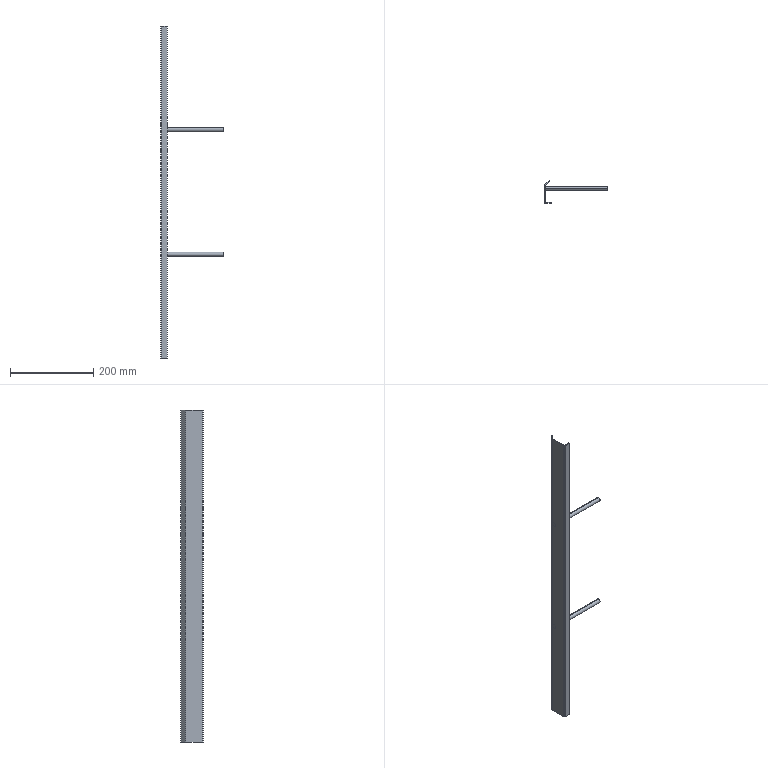Part | STEP file | MM-P41130-12_1 | 1 solid | 20 faces | box 151.5 x 53.167 x 800 mm | volume 109265 mm3 | plane 12 | cylinder 8 | commonest cylinder face diameters 10 x4 1.473 x2 4.473 x2
STEP:
#1=CARTESIAN_POINT('',(0.,0.,0.));
#2=DIRECTION('',(0.,0.,1.));
#3=DIRECTION('',(1.,0.,0.));
#4=AXIS2_PLACEMENT_3D('',#1,#2,#3);
#5=CARTESIAN_POINT('',(0.,-16.5,-145.));
#6=VERTEX_POINT('',#5);
#7=CARTESIAN_POINT('',(0.,-16.5,-155.));
#8=VERTEX_POINT('',#7);
#9=CARTESIAN_POINT('',(0.,-16.5,-150.));
#10=DIRECTION('',(-1.,0.,0.));
#11=DIRECTION('',(0.,0.,-1.));
#12=AXIS2_PLACEMENT_3D('',#9,#10,#11);
#13=CIRCLE('',#12,5.);
#14=CARTESIAN_POINT('',(150.,-16.5,-150.));
#15=DIRECTION('',(1.,0.,0.));
#16=DIRECTION('',(0.,0.,-1.));
#17=AXIS2_PLACEMENT_3D('',#14,#15,#16);
#18=CYLINDRICAL_SURFACE('',#17,5.);
#19=CARTESIAN_POINT('',(6.283,-150.));
#20=DIRECTION('',(-1.,0.));
#21=VECTOR('',#20,1.);
#22=LINE('',#19,#21);
#23=(GEOMETRIC_REPRESENTATION_CONTEXT(2)PARAMETRIC_REPRESENTATION_CONTEXT()REPRESENTATION_CONTEXT('',''));
#24=DEFINITIONAL_REPRESENTATION('',(#22),#23);
#25=PCURVE('',#18,#24);
#26=CARTESIAN_POINT('',(0.,-50.,-400.));
#27=DIRECTION('',(1.,0.,0.));
#28=DIRECTION('',(0.,0.,-1.));
#29=AXIS2_PLACEMENT_3D('',#26,#27,#28);
#30=PLANE('',#29);
#31=CARTESIAN_POINT('',(-245.,33.5));
#32=CARTESIAN_POINT('',(-245.,24.84));
#33=CARTESIAN_POINT('',(-252.5,29.17));
#34=CARTESIAN_POINT('',(-260.,33.5));
#35=CARTESIAN_POINT('',(-252.5,37.83));
#36=CARTESIAN_POINT('',(-245.,42.16));
#37=CARTESIAN_POINT('',(-245.,33.5));
#38=(BOUNDED_CURVE()B_SPLINE_CURVE(2,(#31,#32,#33,#34,#35,#36,#37),.UNSPECIFIED.,.T.,.F.)B_SPLINE_CURVE_WITH_KNOTS((1,2,2,2,2,1),(-2.094,0.,2.094,4.189,6.283,8.378),.UNSPECIFIED.)CURVE()GEOMETRIC_REPRESENTATION_ITEM()RATIONAL_B_SPLINE_CURVE((1.,0.5,1.,0.5,1.,0.5,1.))REPRESENTATION_ITEM(''));
#39=(GEOMETRIC_REPRESENTATION_CONTEXT(2)PARAMETRIC_REPRESENTATION_CONTEXT()REPRESENTATION_CONTEXT('',''));
#40=DEFINITIONAL_REPRESENTATION('',(#38),#39);
#41=PCURVE('',#30,#40);
#42=SURFACE_CURVE('',#13,(#25,#41),.PCURVE_S1.);
#43=EDGE_CURVE('',#6,#8,#42,.T.);
#44=ORIENTED_EDGE('',*,*,#43,.F.);
#45=CARTESIAN_POINT('',(150.,-16.5,-145.));
#46=VERTEX_POINT('',#45);
#47=CARTESIAN_POINT('',(150.,-16.5,-145.));
#48=DIRECTION('',(1.,0.,0.));
#49=VECTOR('',#48,1.);
#50=LINE('',#47,#49);
#51=CARTESIAN_POINT('',(3.142,0.));
#52=DIRECTION('',(0.,1.));
#53=VECTOR('',#52,1.);
#54=LINE('',#51,#53);
#55=(GEOMETRIC_REPRESENTATION_CONTEXT(2)PARAMETRIC_REPRESENTATION_CONTEXT()REPRESENTATION_CONTEXT('',''));
#56=DEFINITIONAL_REPRESENTATION('',(#54),#55);
#57=PCURVE('',#18,#56);
#58=CARTESIAN_POINT('',(150.,-16.5,-150.));
#59=DIRECTION('',(1.,0.,0.));
#60=DIRECTION('',(0.,0.,-1.));
#61=AXIS2_PLACEMENT_3D('',#58,#59,#60);
#62=CYLINDRICAL_SURFACE('',#61,5.);
#63=CARTESIAN_POINT('',(3.142,0.));
#64=DIRECTION('',(0.,1.));
#65=VECTOR('',#64,1.);
#66=LINE('',#63,#65);
#67=(GEOMETRIC_REPRESENTATION_CONTEXT(2)PARAMETRIC_REPRESENTATION_CONTEXT()REPRESENTATION_CONTEXT('',''));
#68=DEFINITIONAL_REPRESENTATION('',(#66),#67);
#69=PCURVE('',#62,#68);
#70=SURFACE_CURVE('',#50,(#57,#69),.PCURVE_S1.);
#71=EDGE_CURVE('',#6,#46,#70,.T.);
#72=ORIENTED_EDGE('',*,*,#71,.T.);
#73=CARTESIAN_POINT('',(150.,-16.5,-155.));
#74=VERTEX_POINT('',#73);
#75=CARTESIAN_POINT('',(150.,-16.5,-150.));
#76=DIRECTION('',(-1.,0.,0.));
#77=DIRECTION('',(0.,0.,-1.));
#78=AXIS2_PLACEMENT_3D('',#75,#76,#77);
#79=CIRCLE('',#78,5.);
#80=CARTESIAN_POINT('',(6.283,0.));
#81=DIRECTION('',(-1.,0.));
#82=VECTOR('',#81,1.);
#83=LINE('',#80,#82);
#84=(GEOMETRIC_REPRESENTATION_CONTEXT(2)PARAMETRIC_REPRESENTATION_CONTEXT()REPRESENTATION_CONTEXT('',''));
#85=DEFINITIONAL_REPRESENTATION('',(#83),#84);
#86=PCURVE('',#18,#85);
#87=CARTESIAN_POINT('',(150.,-16.5,-150.));
#88=DIRECTION('',(1.,0.,0.));
#89=DIRECTION('',(0.,1.,0.));
#90=AXIS2_PLACEMENT_3D('',#87,#88,#89);
#91=PLANE('',#90);
#92=CARTESIAN_POINT('',(0.,-5.));
#93=CARTESIAN_POINT('',(-8.66,-5.));
#94=CARTESIAN_POINT('',(-4.33,2.5));
#95=CARTESIAN_POINT('',(0.,10.));
#96=CARTESIAN_POINT('',(4.33,2.5));
#97=CARTESIAN_POINT('',(8.66,-5.));
#98=CARTESIAN_POINT('',(0.,-5.));
#99=(BOUNDED_CURVE()B_SPLINE_CURVE(2,(#92,#93,#94,#95,#96,#97,#98),.UNSPECIFIED.,.T.,.F.)B_SPLINE_CURVE_WITH_KNOTS((1,2,2,2,2,1),(-2.094,0.,2.094,4.189,6.283,8.378),.UNSPECIFIED.)CURVE()GEOMETRIC_REPRESENTATION_ITEM()RATIONAL_B_SPLINE_CURVE((1.,0.5,1.,0.5,1.,0.5,1.))REPRESENTATION_ITEM(''));
#100=(GEOMETRIC_REPRESENTATION_CONTEXT(2)PARAMETRIC_REPRESENTATION_CONTEXT()REPRESENTATION_CONTEXT('',''));
#101=DEFINITIONAL_REPRESENTATION('',(#99),#100);
#102=PCURVE('',#91,#101);
#103=SURFACE_CURVE('',#79,(#86,#102),.PCURVE_S1.);
#104=EDGE_CURVE('',#46,#74,#103,.T.);
#105=ORIENTED_EDGE('',*,*,#104,.T.);
#106=CARTESIAN_POINT('',(150.,-16.5,-155.));
#107=DIRECTION('',(1.,0.,0.));
#108=VECTOR('',#107,1.);
#109=LINE('',#106,#108);
#110=CARTESIAN_POINT('',(0.,0.));
#111=DIRECTION('',(0.,1.));
#112=VECTOR('',#111,1.);
#113=LINE('',#110,#112);
#114=(GEOMETRIC_REPRESENTATION_CONTEXT(2)PARAMETRIC_REPRESENTATION_CONTEXT()REPRESENTATION_CONTEXT('',''));
#115=DEFINITIONAL_REPRESENTATION('',(#113),#114);
#116=PCURVE('',#18,#115);
#117=CARTESIAN_POINT('',(6.283,0.));
#118=DIRECTION('',(0.,1.));
#119=VECTOR('',#118,1.);
#120=LINE('',#117,#119);
#121=(GEOMETRIC_REPRESENTATION_CONTEXT(2)PARAMETRIC_REPRESENTATION_CONTEXT()REPRESENTATION_CONTEXT('',''));
#122=DEFINITIONAL_REPRESENTATION('',(#120),#121);
#123=PCURVE('',#62,#122);
#124=SURFACE_CURVE('',#109,(#116,#123),.PCURVE_S1.);
#125=EDGE_CURVE('',#8,#74,#124,.T.);
#126=ORIENTED_EDGE('',*,*,#125,.F.);
#127=EDGE_LOOP('',(#44,#72,#105,#126));
#128=FACE_BOUND('',#127,.T.);
#129=ADVANCED_FACE('',(#128),#18,.T.);
#130=CARTESIAN_POINT('',(0.,-16.5,155.));
#131=VERTEX_POINT('',#130);
#132=CARTESIAN_POINT('',(0.,-16.5,145.));
#133=VERTEX_POINT('',#132);
#134=CARTESIAN_POINT('',(0.,-16.5,150.));
#135=DIRECTION('',(-1.,0.,0.));
#136=DIRECTION('',(0.,0.,-1.));
#137=AXIS2_PLACEMENT_3D('',#134,#135,#136);
#138=CIRCLE('',#137,5.);
#139=CARTESIAN_POINT('',(150.,-16.5,150.));
#140=DIRECTION('',(1.,0.,0.));
#141=DIRECTION('',(0.,0.,-1.));
#142=AXIS2_PLACEMENT_3D('',#139,#140,#141);
#143=CYLINDRICAL_SURFACE('',#142,5.);
#144=CARTESIAN_POINT('',(6.283,-150.));
#145=DIRECTION('',(-1.,0.));
#146=VECTOR('',#145,1.);
#147=LINE('',#144,#146);
#148=(GEOMETRIC_REPRESENTATION_CONTEXT(2)PARAMETRIC_REPRESENTATION_CONTEXT()REPRESENTATION_CONTEXT('',''));
#149=DEFINITIONAL_REPRESENTATION('',(#147),#148);
#150=PCURVE('',#143,#149);
#151=CARTESIAN_POINT('',(-545.,33.5));
#152=CARTESIAN_POINT('',(-545.,24.84));
#153=CARTESIAN_POINT('',(-552.5,29.17));
#154=CARTESIAN_POINT('',(-560.,33.5));
#155=CARTESIAN_POINT('',(-552.5,37.83));
#156=CARTESIAN_POINT('',(-545.,42.16));
#157=CARTESIAN_POINT('',(-545.,33.5));
#158=(BOUNDED_CURVE()B_SPLINE_CURVE(2,(#151,#152,#153,#154,#155,#156,#157),.UNSPECIFIED.,.T.,.F.)B_SPLINE_CURVE_WITH_KNOTS((1,2,2,2,2,1),(-2.094,0.,2.094,4.189,6.283,8.378),.UNSPECIFIED.)CURVE()GEOMETRIC_REPRESENTATION_ITEM()RATIONAL_B_SPLINE_CURVE((1.,0.5,1.,0.5,1.,0.5,1.))REPRESENTATION_ITEM(''));
#159=(GEOMETRIC_REPRESENTATION_CONTEXT(2)PARAMETRIC_REPRESENTATION_CONTEXT()REPRESENTATION_CONTEXT('',''));
#160=DEFINITIONAL_REPRESENTATION('',(#158),#159);
#161=PCURVE('',#30,#160);
#162=SURFACE_CURVE('',#138,(#150,#161),.PCURVE_S1.);
#163=EDGE_CURVE('',#131,#133,#162,.T.);
#164=ORIENTED_EDGE('',*,*,#163,.F.);
#165=CARTESIAN_POINT('',(150.,-16.5,155.));
#166=VERTEX_POINT('',#165);
#167=CARTESIAN_POINT('',(150.,-16.5,155.));
#168=DIRECTION('',(1.,0.,0.));
#169=VECTOR('',#168,1.);
#170=LINE('',#167,#169);
#171=CARTESIAN_POINT('',(3.142,0.));
#172=DIRECTION('',(0.,1.));
#173=VECTOR('',#172,1.);
#174=LINE('',#171,#173);
#175=(GEOMETRIC_REPRESENTATION_CONTEXT(2)PARAMETRIC_REPRESENTATION_CONTEXT()REPRESENTATION_CONTEXT('',''));
#176=DEFINITIONAL_REPRESENTATION('',(#174),#175);
#177=PCURVE('',#143,#176);
#178=CARTESIAN_POINT('',(150.,-16.5,150.));
#179=DIRECTION('',(1.,0.,0.));
#180=DIRECTION('',(0.,0.,-1.));
#181=AXIS2_PLACEMENT_3D('',#178,#179,#180);
#182=CYLINDRICAL_SURFACE('',#181,5.);
#183=CARTESIAN_POINT('',(3.142,0.));
#184=DIRECTION('',(0.,1.));
#185=VECTOR('',#184,1.);
#186=LINE('',#183,#185);
#187=(GEOMETRIC_REPRESENTATION_CONTEXT(2)PARAMETRIC_REPRESENTATION_CONTEXT()REPRESENTATION_CONTEXT('',''));
#188=DEFINITIONAL_REPRESENTATION('',(#186),#187);
#189=PCURVE('',#182,#188);
#190=SURFACE_CURVE('',#170,(#177,#189),.PCURVE_S1.);
#191=EDGE_CURVE('',#131,#166,#190,.T.);
#192=ORIENTED_EDGE('',*,*,#191,.T.);
#193=CARTESIAN_POINT('',(150.,-16.5,145.));
#194=VERTEX_POINT('',#193);
#195=CARTESIAN_POINT('',(150.,-16.5,150.));
#196=DIRECTION('',(-1.,0.,0.));
#197=DIRECTION('',(0.,0.,-1.));
#198=AXIS2_PLACEMENT_3D('',#195,#196,#197);
#199=CIRCLE('',#198,5.);
#200=CARTESIAN_POINT('',(6.283,0.));
#201=DIRECTION('',(-1.,0.));
#202=VECTOR('',#201,1.);
#203=LINE('',#200,#202);
#204=(GEOMETRIC_REPRESENTATION_CONTEXT(2)PARAMETRIC_REPRESENTATION_CONTEXT()REPRESENTATION_CONTEXT('',''));
#205=DEFINITIONAL_REPRESENTATION('',(#203),#204);
#206=PCURVE('',#143,#205);
#207=CARTESIAN_POINT('',(150.,-16.5,150.));
#208=DIRECTION('',(1.,0.,0.));
#209=DIRECTION('',(0.,1.,0.));
#210=AXIS2_PLACEMENT_3D('',#207,#208,#209);
#211=PLANE('',#210);
#212=CARTESIAN_POINT('',(0.,-5.));
#213=CARTESIAN_POINT('',(-8.66,-5.));
#214=CARTESIAN_POINT('',(-4.33,2.5));
#215=CARTESIAN_POINT('',(0.,10.));
#216=CARTESIAN_POINT('',(4.33,2.5));
#217=CARTESIAN_POINT('',(8.66,-5.));
#218=CARTESIAN_POINT('',(0.,-5.));
#219=(BOUNDED_CURVE()B_SPLINE_CURVE(2,(#212,#213,#214,#215,#216,#217,#218),.UNSPECIFIED.,.T.,.F.)B_SPLINE_CURVE_WITH_KNOTS((1,2,2,2,2,1),(-2.094,0.,2.094,4.189,6.283,8.378),.UNSPECIFIED.)CURVE()GEOMETRIC_REPRESENTATION_ITEM()RATIONAL_B_SPLINE_CURVE((1.,0.5,1.,0.5,1.,0.5,1.))REPRESENTATION_ITEM(''));
#220=(GEOMETRIC_REPRESENTATION_CONTEXT(2)PARAMETRIC_REPRESENTATION_CONTEXT()REPRESENTATION_CONTEXT('',''));
#221=DEFINITIONAL_REPRESENTATION('',(#219),#220);
#222=PCURVE('',#211,#221);
#223=SURFACE_CURVE('',#199,(#206,#222),.PCURVE_S1.);
#224=EDGE_CURVE('',#166,#194,#223,.T.);
#225=ORIENTED_EDGE('',*,*,#224,.T.);
#226=CARTESIAN_POINT('',(150.,-16.5,145.));
#227=DIRECTION('',(1.,0.,0.));
#228=VECTOR('',#227,1.);
#229=LINE('',#226,#228);
#230=CARTESIAN_POINT('',(0.,0.));
#231=DIRECTION('',(0.,1.));
#232=VECTOR('',#231,1.);
#233=LINE('',#230,#232);
#234=(GEOMETRIC_REPRESENTATION_CONTEXT(2)PARAMETRIC_REPRESENTATION_CONTEXT()REPRESENTATION_CONTEXT('',''));
#235=DEFINITIONAL_REPRESENTATION('',(#233),#234);
#236=PCURVE('',#143,#235);
#237=CARTESIAN_POINT('',(6.283,0.));
#238=DIRECTION('',(0.,1.));
#239=VECTOR('',#238,1.);
#240=LINE('',#237,#239);
#241=(GEOMETRIC_REPRESENTATION_CONTEXT(2)PARAMETRIC_REPRESENTATION_CONTEXT()REPRESENTATION_CONTEXT('',''));
#242=DEFINITIONAL_REPRESENTATION('',(#240),#241);
#243=PCURVE('',#182,#242);
#244=SURFACE_CURVE('',#229,(#236,#243),.PCURVE_S1.);
#245=EDGE_CURVE('',#133,#194,#244,.T.);
#246=ORIENTED_EDGE('',*,*,#245,.F.);
#247=EDGE_LOOP('',(#164,#192,#225,#246));
#248=FACE_BOUND('',#247,.T.);
#249=ADVANCED_FACE('',(#248),#143,.T.);
#250=CARTESIAN_POINT('',(-1.5,-10.305,-400.));
#251=VERTEX_POINT('',#250);
#252=CARTESIAN_POINT('',(-1.5,-10.305,400.));
#253=VERTEX_POINT('',#252);
#254=CARTESIAN_POINT('',(-1.5,-10.305,-400.));
#255=DIRECTION('',(0.,0.,1.));
#256=VECTOR('',#255,1.);
#257=LINE('',#254,#256);
#258=CARTESIAN_POINT('',(-1.5,-50.,-400.));
#259=DIRECTION('',(1.,0.,0.));
#260=DIRECTION('',(0.,0.,-1.));
#261=AXIS2_PLACEMENT_3D('',#258,#259,#260);
#262=PLANE('',#261);
#263=CARTESIAN_POINT('',(0.,39.695));
#264=DIRECTION('',(-1.,0.));
#265=VECTOR('',#264,1.);
#266=LINE('',#263,#265);
#267=(GEOMETRIC_REPRESENTATION_CONTEXT(2)PARAMETRIC_REPRESENTATION_CONTEXT()REPRESENTATION_CONTEXT('',''));
#268=DEFINITIONAL_REPRESENTATION('',(#266),#267);
#269=PCURVE('',#262,#268);
#270=CARTESIAN_POINT('',(0.7366,-10.305,-400.));
#271=DIRECTION('',(0.,0.,-1.));
#272=DIRECTION('',(-1.,0.,0.));
#273=AXIS2_PLACEMENT_3D('',#270,#271,#272);
#274=CYLINDRICAL_SURFACE('',#273,2.237);
#275=CARTESIAN_POINT('',(0.,0.));
#276=DIRECTION('',(0.,-1.));
#277=VECTOR('',#276,1.);
#278=LINE('',#275,#277);
#279=(GEOMETRIC_REPRESENTATION_CONTEXT(2)PARAMETRIC_REPRESENTATION_CONTEXT()REPRESENTATION_CONTEXT('',''));
#280=DEFINITIONAL_REPRESENTATION('',(#278),#279);
#281=PCURVE('',#274,#280);
#282=SURFACE_CURVE('',#257,(#269,#281),.PCURVE_S1.);
#283=EDGE_CURVE('',#251,#253,#282,.T.);
#284=ORIENTED_EDGE('',*,*,#283,.F.);
#285=CARTESIAN_POINT('',(-1.5,-49.263,-400.));
#286=VERTEX_POINT('',#285);
#287=CARTESIAN_POINT('',(-1.5,-50.,-400.));
#288=DIRECTION('',(0.,1.,0.));
#289=VECTOR('',#288,1.);
#290=LINE('',#287,#289);
#291=CARTESIAN_POINT('',(0.,0.));
#292=DIRECTION('',(0.,1.));
#293=VECTOR('',#292,1.);
#294=LINE('',#291,#293);
#295=(GEOMETRIC_REPRESENTATION_CONTEXT(2)PARAMETRIC_REPRESENTATION_CONTEXT()REPRESENTATION_CONTEXT('',''));
#296=DEFINITIONAL_REPRESENTATION('',(#294),#295);
#297=PCURVE('',#262,#296);
#298=CARTESIAN_POINT('',(0.,-49.263,-400.));
#299=DIRECTION('',(0.,0.,-1.));
#300=DIRECTION('',(-1.,0.,0.));
#301=AXIS2_PLACEMENT_3D('',#298,#299,#300);
#302=PLANE('',#301);
#303=CARTESIAN_POINT('',(1.5,-0.7366));
#304=DIRECTION('',(0.,1.));
#305=VECTOR('',#304,1.);
#306=LINE('',#303,#305);
#307=(GEOMETRIC_REPRESENTATION_CONTEXT(2)PARAMETRIC_REPRESENTATION_CONTEXT()REPRESENTATION_CONTEXT('',''));
#308=DEFINITIONAL_REPRESENTATION('',(#306),#307);
#309=PCURVE('',#302,#308);
#310=SURFACE_CURVE('',#290,(#297,#309),.PCURVE_S1.);
#311=EDGE_CURVE('',#286,#251,#310,.T.);
#312=ORIENTED_EDGE('',*,*,#311,.F.);
#313=CARTESIAN_POINT('',(-1.5,-49.263,400.));
#314=VERTEX_POINT('',#313);
#315=CARTESIAN_POINT('',(-1.5,-49.263,-400.));
#316=DIRECTION('',(0.,0.,-1.));
#317=VECTOR('',#316,1.);
#318=LINE('',#315,#317);
#319=CARTESIAN_POINT('',(0.,0.7366));
#320=DIRECTION('',(1.,0.));
#321=VECTOR('',#320,1.);
#322=LINE('',#319,#321);
#323=(GEOMETRIC_REPRESENTATION_CONTEXT(2)PARAMETRIC_REPRESENTATION_CONTEXT()REPRESENTATION_CONTEXT('',''));
#324=DEFINITIONAL_REPRESENTATION('',(#322),#323);
#325=PCURVE('',#262,#324);
#326=CARTESIAN_POINT('',(0.7366,-49.263,-400.));
#327=DIRECTION('',(0.,0.,-1.));
#328=DIRECTION('',(-1.,0.,0.));
#329=AXIS2_PLACEMENT_3D('',#326,#327,#328);
#330=CYLINDRICAL_SURFACE('',#329,2.237);
#331=CARTESIAN_POINT('',(6.283,0.));
#332=DIRECTION('',(0.,1.));
#333=VECTOR('',#332,1.);
#334=LINE('',#331,#333);
#335=(GEOMETRIC_REPRESENTATION_CONTEXT(2)PARAMETRIC_REPRESENTATION_CONTEXT()REPRESENTATION_CONTEXT('',''));
#336=DEFINITIONAL_REPRESENTATION('',(#334),#335);
#337=PCURVE('',#330,#336);
#338=SURFACE_CURVE('',#318,(#325,#337),.PCURVE_S1.);
#339=EDGE_CURVE('',#314,#286,#338,.T.);
#340=ORIENTED_EDGE('',*,*,#339,.F.);
#341=CARTESIAN_POINT('',(-1.5,-50.,400.));
#342=DIRECTION('',(0.,-1.,0.));
#343=VECTOR('',#342,1.);
#344=LINE('',#341,#343);
#345=CARTESIAN_POINT('',(-800.,0.));
#346=DIRECTION('',(0.,-1.));
#347=VECTOR('',#346,1.);
#348=LINE('',#345,#347);
#349=(GEOMETRIC_REPRESENTATION_CONTEXT(2)PARAMETRIC_REPRESENTATION_CONTEXT()REPRESENTATION_CONTEXT('',''));
#350=DEFINITIONAL_REPRESENTATION('',(#348),#349);
#351=PCURVE('',#262,#350);
#352=CARTESIAN_POINT('',(0.,-10.305,400.));
#353=DIRECTION('',(0.,0.,1.));
#354=DIRECTION('',(1.,0.,0.));
#355=AXIS2_PLACEMENT_3D('',#352,#353,#354);
#356=PLANE('',#355);
#357=CARTESIAN_POINT('',(-1.5,-39.695));
#358=DIRECTION('',(0.,-1.));
#359=VECTOR('',#358,1.);
#360=LINE('',#357,#359);
#361=(GEOMETRIC_REPRESENTATION_CONTEXT(2)PARAMETRIC_REPRESENTATION_CONTEXT()REPRESENTATION_CONTEXT('',''));
#362=DEFINITIONAL_REPRESENTATION('',(#360),#361);
#363=PCURVE('',#356,#362);
#364=SURFACE_CURVE('',#344,(#351,#363),.PCURVE_S1.);
#365=EDGE_CURVE('',#253,#314,#364,.T.);
#366=ORIENTED_EDGE('',*,*,#365,.F.);
#367=EDGE_LOOP('',(#284,#312,#340,#366));
#368=FACE_BOUND('',#367,.T.);
#369=ADVANCED_FACE('',(#368),#262,.F.);
#370=CARTESIAN_POINT('',(10.607,0.6066,400.));
#371=VERTEX_POINT('',#370);
#372=CARTESIAN_POINT('',(9.546,1.667,400.));
#373=VERTEX_POINT('',#372);
#374=CARTESIAN_POINT('',(9.546,1.667,400.));
#375=DIRECTION('',(-0.7071,0.7071,0.));
#376=VECTOR('',#375,1.);
#377=LINE('',#374,#376);
#378=CARTESIAN_POINT('',(9.546,11.972));
#379=DIRECTION('',(-0.7071,0.7071));
#380=VECTOR('',#379,1.);
#381=LINE('',#378,#380);
#382=(GEOMETRIC_REPRESENTATION_CONTEXT(2)PARAMETRIC_REPRESENTATION_CONTEXT()REPRESENTATION_CONTEXT('',''));
#383=DEFINITIONAL_REPRESENTATION('',(#381),#382);
#384=PCURVE('',#356,#383);
#385=CARTESIAN_POINT('',(9.546,1.667,-400.));
#386=DIRECTION('',(-0.7071,-0.7071,0.));
#387=DIRECTION('',(0.7071,-0.7071,0.));
#388=AXIS2_PLACEMENT_3D('',#385,#386,#387);
#389=PLANE('',#388);
#390=CARTESIAN_POINT('',(0.,800.));
#391=DIRECTION('',(-1.,0.));
#392=VECTOR('',#391,1.);
#393=LINE('',#390,#392);
#394=(GEOMETRIC_REPRESENTATION_CONTEXT(2)PARAMETRIC_REPRESENTATION_CONTEXT()REPRESENTATION_CONTEXT('',''));
#395=DEFINITIONAL_REPRESENTATION('',(#393),#394);
#396=PCURVE('',#389,#395);
#397=SURFACE_CURVE('',#377,(#384,#396),.PCURVE_S1.);
#398=EDGE_CURVE('',#371,#373,#397,.T.);
#399=ORIENTED_EDGE('',*,*,#398,.T.);
#400=CARTESIAN_POINT('',(-0.8449,-8.724,400.));
#401=VERTEX_POINT('',#400);
#402=CARTESIAN_POINT('',(9.546,1.667,400.));
#403=DIRECTION('',(-0.7071,-0.7071,0.));
#404=VECTOR('',#403,1.);
#405=LINE('',#402,#404);
#406=CARTESIAN_POINT('',(9.546,11.972));
#407=DIRECTION('',(-0.7071,-0.7071));
#408=VECTOR('',#407,1.);
#409=LINE('',#406,#408);
#410=(GEOMETRIC_REPRESENTATION_CONTEXT(2)PARAMETRIC_REPRESENTATION_CONTEXT()REPRESENTATION_CONTEXT('',''));
#411=DEFINITIONAL_REPRESENTATION('',(#409),#410);
#412=PCURVE('',#356,#411);
#413=CARTESIAN_POINT('',(-1.061,-8.939,-400.));
#414=DIRECTION('',(0.7071,-0.7071,0.));
#415=DIRECTION('',(0.7071,0.7071,0.));
#416=AXIS2_PLACEMENT_3D('',#413,#414,#415);
#417=PLANE('',#416);
#418=CARTESIAN_POINT('',(15.,800.));
#419=DIRECTION('',(-1.,0.));
#420=VECTOR('',#419,1.);
#421=LINE('',#418,#420);
#422=(GEOMETRIC_REPRESENTATION_CONTEXT(2)PARAMETRIC_REPRESENTATION_CONTEXT()REPRESENTATION_CONTEXT('',''));
#423=DEFINITIONAL_REPRESENTATION('',(#421),#422);
#424=PCURVE('',#417,#423);
#425=SURFACE_CURVE('',#405,(#412,#424),.PCURVE_S1.);
#426=EDGE_CURVE('',#373,#401,#425,.T.);
#427=ORIENTED_EDGE('',*,*,#426,.T.);
#428=CARTESIAN_POINT('',(0.7366,-10.305,400.));
#429=DIRECTION('',(0.,0.,1.));
#430=DIRECTION('',(-1.,0.,0.));
#431=AXIS2_PLACEMENT_3D('',#428,#429,#430);
#432=CIRCLE('',#431,2.237);
#433=CARTESIAN_POINT('',(0.7366,0.));
#434=DIRECTION('',(-1.,0.));
#435=AXIS2_PLACEMENT_2D('',#433,#434);
#436=CIRCLE('',#435,2.237);
#437=(GEOMETRIC_REPRESENTATION_CONTEXT(2)PARAMETRIC_REPRESENTATION_CONTEXT()REPRESENTATION_CONTEXT('',''));
#438=DEFINITIONAL_REPRESENTATION('',(#436),#437);
#439=PCURVE('',#356,#438);
#440=CARTESIAN_POINT('',(6.283,-800.));
#441=DIRECTION('',(-1.,0.));
#442=VECTOR('',#441,1.);
#443=LINE('',#440,#442);
#444=(GEOMETRIC_REPRESENTATION_CONTEXT(2)PARAMETRIC_REPRESENTATION_CONTEXT()REPRESENTATION_CONTEXT('',''));
#445=DEFINITIONAL_REPRESENTATION('',(#443),#444);
#446=PCURVE('',#274,#445);
#447=SURFACE_CURVE('',#432,(#439,#446),.PCURVE_S1.);
#448=EDGE_CURVE('',#401,#253,#447,.T.);
#449=ORIENTED_EDGE('',*,*,#448,.T.);
#450=ORIENTED_EDGE('',*,*,#365,.T.);
#451=CARTESIAN_POINT('',(0.7366,-51.5,400.));
#452=VERTEX_POINT('',#451);
#453=CARTESIAN_POINT('',(0.7366,-49.263,400.));
#454=DIRECTION('',(0.,0.,1.));
#455=DIRECTION('',(-1.,0.,0.));
#456=AXIS2_PLACEMENT_3D('',#453,#454,#455);
#457=CIRCLE('',#456,2.237);
#458=CARTESIAN_POINT('',(0.7366,-38.958));
#459=DIRECTION('',(-1.,0.));
#460=AXIS2_PLACEMENT_2D('',#458,#459);
#461=CIRCLE('',#460,2.237);
#462=(GEOMETRIC_REPRESENTATION_CONTEXT(2)PARAMETRIC_REPRESENTATION_CONTEXT()REPRESENTATION_CONTEXT('',''));
#463=DEFINITIONAL_REPRESENTATION('',(#461),#462);
#464=PCURVE('',#356,#463);
#465=CARTESIAN_POINT('',(6.283,-800.));
#466=DIRECTION('',(-1.,0.));
#467=VECTOR('',#466,1.);
#468=LINE('',#465,#467);
#469=(GEOMETRIC_REPRESENTATION_CONTEXT(2)PARAMETRIC_REPRESENTATION_CONTEXT()REPRESENTATION_CONTEXT('',''));
#470=DEFINITIONAL_REPRESENTATION('',(#468),#469);
#471=PCURVE('',#330,#470);
#472=SURFACE_CURVE('',#457,(#464,#471),.PCURVE_S1.);
#473=EDGE_CURVE('',#314,#452,#472,.T.);
#474=ORIENTED_EDGE('',*,*,#473,.T.);
#475=CARTESIAN_POINT('',(15.,-51.5,400.));
#476=VERTEX_POINT('',#475);
#477=CARTESIAN_POINT('',(0.,-51.5,400.));
#478=DIRECTION('',(1.,0.,0.));
#479=VECTOR('',#478,1.);
#480=LINE('',#477,#479);
#481=CARTESIAN_POINT('',(0.,-41.195));
#482=DIRECTION('',(1.,0.));
#483=VECTOR('',#482,1.);
#484=LINE('',#481,#483);
#485=(GEOMETRIC_REPRESENTATION_CONTEXT(2)PARAMETRIC_REPRESENTATION_CONTEXT()REPRESENTATION_CONTEXT('',''));
#486=DEFINITIONAL_REPRESENTATION('',(#484),#485);
#487=PCURVE('',#356,#486);
#488=CARTESIAN_POINT('',(0.,-51.5,-400.));
#489=DIRECTION('',(0.,1.,0.));
#490=DIRECTION('',(0.,0.,1.));
#491=AXIS2_PLACEMENT_3D('',#488,#489,#490);
#492=PLANE('',#491);
#493=CARTESIAN_POINT('',(800.,0.));
#494=DIRECTION('',(0.,1.));
#495=VECTOR('',#494,1.);
#496=LINE('',#493,#495);
#497=(GEOMETRIC_REPRESENTATION_CONTEXT(2)PARAMETRIC_REPRESENTATION_CONTEXT()REPRESENTATION_CONTEXT('',''));
#498=DEFINITIONAL_REPRESENTATION('',(#496),#497);
#499=PCURVE('',#492,#498);
#500=SURFACE_CURVE('',#480,(#487,#499),.PCURVE_S1.);
#501=EDGE_CURVE('',#452,#476,#500,.T.);
#502=ORIENTED_EDGE('',*,*,#501,.T.);
#503=CARTESIAN_POINT('',(15.,-50.,400.));
#504=VERTEX_POINT('',#503);
#505=CARTESIAN_POINT('',(15.,-50.,400.));
#506=DIRECTION('',(0.,1.,0.));
#507=VECTOR('',#506,1.);
#508=LINE('',#505,#507);
#509=CARTESIAN_POINT('',(15.,-39.695));
#510=DIRECTION('',(0.,1.));
#511=VECTOR('',#510,1.);
#512=LINE('',#509,#511);
#513=(GEOMETRIC_REPRESENTATION_CONTEXT(2)PARAMETRIC_REPRESENTATION_CONTEXT()REPRESENTATION_CONTEXT('',''));
#514=DEFINITIONAL_REPRESENTATION('',(#512),#513);
#515=PCURVE('',#356,#514);
#516=CARTESIAN_POINT('',(15.,-50.,-400.));
#517=DIRECTION('',(-1.,0.,0.));
#518=DIRECTION('',(0.,0.,1.));
#519=AXIS2_PLACEMENT_3D('',#516,#517,#518);
#520=PLANE('',#519);
#521=CARTESIAN_POINT('',(800.,0.));
#522=DIRECTION('',(0.,1.));
#523=VECTOR('',#522,1.);
#524=LINE('',#521,#523);
#525=(GEOMETRIC_REPRESENTATION_CONTEXT(2)PARAMETRIC_REPRESENTATION_CONTEXT()REPRESENTATION_CONTEXT('',''));
#526=DEFINITIONAL_REPRESENTATION('',(#524),#525);
#527=PCURVE('',#520,#526);
#528=SURFACE_CURVE('',#508,(#515,#527),.PCURVE_S1.);
#529=EDGE_CURVE('',#476,#504,#528,.T.);
#530=ORIENTED_EDGE('',*,*,#529,.T.);
#531=CARTESIAN_POINT('',(0.7366,-50.,400.));
#532=VERTEX_POINT('',#531);
#533=CARTESIAN_POINT('',(0.,-50.,400.));
#534=DIRECTION('',(-1.,0.,0.));
#535=VECTOR('',#534,1.);
#536=LINE('',#533,#535);
#537=CARTESIAN_POINT('',(0.,-39.695));
#538=DIRECTION('',(-1.,0.));
#539=VECTOR('',#538,1.);
#540=LINE('',#537,#539);
#541=(GEOMETRIC_REPRESENTATION_CONTEXT(2)PARAMETRIC_REPRESENTATION_CONTEXT()REPRESENTATION_CONTEXT('',''));
#542=DEFINITIONAL_REPRESENTATION('',(#540),#541);
#543=PCURVE('',#356,#542);
#544=CARTESIAN_POINT('',(0.,-50.,-400.));
#545=DIRECTION('',(0.,1.,0.));
#546=DIRECTION('',(0.,0.,1.));
#547=AXIS2_PLACEMENT_3D('',#544,#545,#546);
#548=PLANE('',#547);
#549=CARTESIAN_POINT('',(800.,0.));
#550=DIRECTION('',(0.,-1.));
#551=VECTOR('',#550,1.);
#552=LINE('',#549,#551);
#553=(GEOMETRIC_REPRESENTATION_CONTEXT(2)PARAMETRIC_REPRESENTATION_CONTEXT()REPRESENTATION_CONTEXT('',''));
#554=DEFINITIONAL_REPRESENTATION('',(#552),#553);
#555=PCURVE('',#548,#554);
#556=SURFACE_CURVE('',#536,(#543,#555),.PCURVE_S1.);
#557=EDGE_CURVE('',#504,#532,#556,.T.);
#558=ORIENTED_EDGE('',*,*,#557,.T.);
#559=CARTESIAN_POINT('',(0.,-49.263,400.));
#560=VERTEX_POINT('',#559);
#561=CARTESIAN_POINT('',(0.7366,-49.263,400.));
#562=DIRECTION('',(0.,0.,-1.));
#563=DIRECTION('',(-1.,0.,0.));
#564=AXIS2_PLACEMENT_3D('',#561,#562,#563);
#565=CIRCLE('',#564,0.7366);
#566=CARTESIAN_POINT('',(0.,-38.958));
#567=CARTESIAN_POINT('',(0.,-37.682));
#568=CARTESIAN_POINT('',(1.105,-38.32));
#569=CARTESIAN_POINT('',(2.21,-38.958));
#570=CARTESIAN_POINT('',(1.105,-39.596));
#571=CARTESIAN_POINT('',(0.,-40.234));
#572=CARTESIAN_POINT('',(0.,-38.958));
#573=(BOUNDED_CURVE()B_SPLINE_CURVE(2,(#566,#567,#568,#569,#570,#571,#572),.UNSPECIFIED.,.T.,.F.)B_SPLINE_CURVE_WITH_KNOTS((1,2,2,2,2,1),(-2.094,0.,2.094,4.189,6.283,8.378),.UNSPECIFIED.)CURVE()GEOMETRIC_REPRESENTATION_ITEM()RATIONAL_B_SPLINE_CURVE((1.,0.5,1.,0.5,1.,0.5,1.))REPRESENTATION_ITEM(''));
#574=(GEOMETRIC_REPRESENTATION_CONTEXT(2)PARAMETRIC_REPRESENTATION_CONTEXT()REPRESENTATION_CONTEXT('',''));
#575=DEFINITIONAL_REPRESENTATION('',(#573),#574);
#576=PCURVE('',#356,#575);
#577=CARTESIAN_POINT('',(0.7366,-49.263,-400.));
#578=DIRECTION('',(0.,0.,-1.));
#579=DIRECTION('',(-1.,0.,0.));
#580=AXIS2_PLACEMENT_3D('',#577,#578,#579);
#581=CYLINDRICAL_SURFACE('',#580,0.7366);
#582=CARTESIAN_POINT('',(0.,-800.));
#583=DIRECTION('',(1.,0.));
#584=VECTOR('',#583,1.);
#585=LINE('',#582,#584);
#586=(GEOMETRIC_REPRESENTATION_CONTEXT(2)PARAMETRIC_REPRESENTATION_CONTEXT()REPRESENTATION_CONTEXT('',''));
#587=DEFINITIONAL_REPRESENTATION('',(#585),#586);
#588=PCURVE('',#581,#587);
#589=SURFACE_CURVE('',#565,(#576,#588),.PCURVE_S1.);
#590=EDGE_CURVE('',#532,#560,#589,.T.);
#591=ORIENTED_EDGE('',*,*,#590,.T.);
#592=CARTESIAN_POINT('',(0.,-10.305,400.));
#593=VERTEX_POINT('',#592);
#594=CARTESIAN_POINT('',(0.,-10.305,400.));
#595=DIRECTION('',(0.,1.,0.));
#596=VECTOR('',#595,1.);
#597=LINE('',#594,#596);
#598=CARTESIAN_POINT('',(0.,0.));
#599=DIRECTION('',(0.,1.));
#600=VECTOR('',#599,1.);
#601=LINE('',#598,#600);
#602=(GEOMETRIC_REPRESENTATION_CONTEXT(2)PARAMETRIC_REPRESENTATION_CONTEXT()REPRESENTATION_CONTEXT('',''));
#603=DEFINITIONAL_REPRESENTATION('',(#601),#602);
#604=PCURVE('',#356,#603);
#605=CARTESIAN_POINT('',(-800.,39.695));
#606=DIRECTION('',(0.,1.));
#607=VECTOR('',#606,1.);
#608=LINE('',#605,#607);
#609=(GEOMETRIC_REPRESENTATION_CONTEXT(2)PARAMETRIC_REPRESENTATION_CONTEXT()REPRESENTATION_CONTEXT('',''));
#610=DEFINITIONAL_REPRESENTATION('',(#608),#609);
#611=PCURVE('',#30,#610);
#612=SURFACE_CURVE('',#597,(#604,#611),.PCURVE_S1.);
#613=EDGE_CURVE('',#560,#593,#612,.T.);
#614=ORIENTED_EDGE('',*,*,#613,.T.);
#615=CARTESIAN_POINT('',(0.2157,-9.784,400.));
#616=VERTEX_POINT('',#615);
#617=CARTESIAN_POINT('',(0.7366,-10.305,400.));
#618=DIRECTION('',(0.,0.,-1.));
#619=DIRECTION('',(-1.,0.,0.));
#620=AXIS2_PLACEMENT_3D('',#617,#618,#619);
#621=CIRCLE('',#620,0.7366);
#622=CARTESIAN_POINT('',(0.,0.));
#623=CARTESIAN_POINT('',(0.,1.276));
#624=CARTESIAN_POINT('',(1.105,0.6379));
#625=CARTESIAN_POINT('',(2.21,0.));
#626=CARTESIAN_POINT('',(1.105,-0.6379));
#627=CARTESIAN_POINT('',(0.,-1.276));
#628=CARTESIAN_POINT('',(0.,0.));
#629=(BOUNDED_CURVE()B_SPLINE_CURVE(2,(#622,#623,#624,#625,#626,#627,#628),.UNSPECIFIED.,.T.,.F.)B_SPLINE_CURVE_WITH_KNOTS((1,2,2,2,2,1),(-2.094,0.,2.094,4.189,6.283,8.378),.UNSPECIFIED.)CURVE()GEOMETRIC_REPRESENTATION_ITEM()RATIONAL_B_SPLINE_CURVE((1.,0.5,1.,0.5,1.,0.5,1.))REPRESENTATION_ITEM(''));
#630=(GEOMETRIC_REPRESENTATION_CONTEXT(2)PARAMETRIC_REPRESENTATION_CONTEXT()REPRESENTATION_CONTEXT('',''));
#631=DEFINITIONAL_REPRESENTATION('',(#629),#630);
#632=PCURVE('',#356,#631);
#633=CARTESIAN_POINT('',(0.7366,-10.305,-400.));
#634=DIRECTION('',(0.,0.,-1.));
#635=DIRECTION('',(-1.,0.,0.));
#636=AXIS2_PLACEMENT_3D('',#633,#634,#635);
#637=CYLINDRICAL_SURFACE('',#636,0.7366);
#638=CARTESIAN_POINT('',(0.,-800.));
#639=DIRECTION('',(1.,0.));
#640=VECTOR('',#639,1.);
#641=LINE('',#638,#640);
#642=(GEOMETRIC_REPRESENTATION_CONTEXT(2)PARAMETRIC_REPRESENTATION_CONTEXT()REPRESENTATION_CONTEXT('',''));
#643=DEFINITIONAL_REPRESENTATION('',(#641),#642);
#644=PCURVE('',#637,#643);
#645=SURFACE_CURVE('',#621,(#632,#644),.PCURVE_S1.);
#646=EDGE_CURVE('',#593,#616,#645,.T.);
#647=ORIENTED_EDGE('',*,*,#646,.T.);
#648=CARTESIAN_POINT('',(0.2157,-9.784,400.));
#649=DIRECTION('',(0.7071,0.7071,0.));
#650=VECTOR('',#649,1.);
#651=LINE('',#648,#650);
#652=CARTESIAN_POINT('',(0.2157,0.5209));
#653=DIRECTION('',(0.7071,0.7071));
#654=VECTOR('',#653,1.);
#655=LINE('',#652,#654);
#656=(GEOMETRIC_REPRESENTATION_CONTEXT(2)PARAMETRIC_REPRESENTATION_CONTEXT()REPRESENTATION_CONTEXT('',''));
#657=DEFINITIONAL_REPRESENTATION('',(#655),#656);
#658=PCURVE('',#356,#657);
#659=CARTESIAN_POINT('',(0.,-10.,-400.));
#660=DIRECTION('',(0.7071,-0.7071,0.));
#661=DIRECTION('',(0.7071,0.7071,0.));
#662=AXIS2_PLACEMENT_3D('',#659,#660,#661);
#663=PLANE('',#662);
#664=CARTESIAN_POINT('',(0.3051,800.));
#665=DIRECTION('',(1.,0.));
#666=VECTOR('',#665,1.);
#667=LINE('',#664,#666);
#668=(GEOMETRIC_REPRESENTATION_CONTEXT(2)PARAMETRIC_REPRESENTATION_CONTEXT()REPRESENTATION_CONTEXT('',''));
#669=DEFINITIONAL_REPRESENTATION('',(#667),#668);
#670=PCURVE('',#663,#669);
#671=SURFACE_CURVE('',#651,(#658,#670),.PCURVE_S1.);
#672=EDGE_CURVE('',#616,#371,#671,.T.);
#673=ORIENTED_EDGE('',*,*,#672,.T.);
#674=EDGE_LOOP('',(#399,#427,#449,#450,#474,#502,#530,#558,#591,#614,#647,#673));
#675=FACE_BOUND('',#674,.T.);
#676=ADVANCED_FACE('',(#675),#356,.T.);
#677=CARTESIAN_POINT('',(-0.8449,-8.724,-400.));
#678=VERTEX_POINT('',#677);
#679=CARTESIAN_POINT('',(0.7366,-10.305,-400.));
#680=DIRECTION('',(0.,0.,1.));
#681=DIRECTION('',(-1.,0.,0.));
#682=AXIS2_PLACEMENT_3D('',#679,#680,#681);
#683=CIRCLE('',#682,2.237);
#684=CARTESIAN_POINT('',(6.283,0.));
#685=DIRECTION('',(-1.,0.));
#686=VECTOR('',#685,1.);
#687=LINE('',#684,#686);
#688=(GEOMETRIC_REPRESENTATION_CONTEXT(2)PARAMETRIC_REPRESENTATION_CONTEXT()REPRESENTATION_CONTEXT('',''));
#689=DEFINITIONAL_REPRESENTATION('',(#687),#688);
#690=PCURVE('',#274,#689);
#691=CARTESIAN_POINT('',(1.5,38.958));
#692=CARTESIAN_POINT('',(1.5,35.084));
#693=CARTESIAN_POINT('',(-1.855,37.021));
#694=CARTESIAN_POINT('',(-5.21,38.958));
#695=CARTESIAN_POINT('',(-1.855,40.895));
#696=CARTESIAN_POINT('',(1.5,42.832));
#697=CARTESIAN_POINT('',(1.5,38.958));
#698=(BOUNDED_CURVE()B_SPLINE_CURVE(2,(#691,#692,#693,#694,#695,#696,#697),.UNSPECIFIED.,.T.,.F.)B_SPLINE_CURVE_WITH_KNOTS((1,2,2,2,2,1),(-2.094,0.,2.094,4.189,6.283,8.378),.UNSPECIFIED.)CURVE()GEOMETRIC_REPRESENTATION_ITEM()RATIONAL_B_SPLINE_CURVE((1.,0.5,1.,0.5,1.,0.5,1.))REPRESENTATION_ITEM(''));
#699=(GEOMETRIC_REPRESENTATION_CONTEXT(2)PARAMETRIC_REPRESENTATION_CONTEXT()REPRESENTATION_CONTEXT('',''));
#700=DEFINITIONAL_REPRESENTATION('',(#698),#699);
#701=PCURVE('',#302,#700);
#702=SURFACE_CURVE('',#683,(#690,#701),.PCURVE_S1.);
#703=EDGE_CURVE('',#678,#251,#702,.T.);
#704=ORIENTED_EDGE('',*,*,#703,.T.);
#705=ORIENTED_EDGE('',*,*,#283,.T.);
#706=ORIENTED_EDGE('',*,*,#448,.F.);
#707=CARTESIAN_POINT('',(-0.8449,-8.724,-400.));
#708=DIRECTION('',(0.,0.,-1.));
#709=VECTOR('',#708,1.);
#710=LINE('',#707,#709);
#711=CARTESIAN_POINT('',(0.7854,0.));
#712=DIRECTION('',(0.,1.));
#713=VECTOR('',#712,1.);
#714=LINE('',#711,#713);
#715=(GEOMETRIC_REPRESENTATION_CONTEXT(2)PARAMETRIC_REPRESENTATION_CONTEXT()REPRESENTATION_CONTEXT('',''));
#716=DEFINITIONAL_REPRESENTATION('',(#714),#715);
#717=PCURVE('',#274,#716);
#718=CARTESIAN_POINT('',(0.3051,0.));
#719=DIRECTION('',(0.,-1.));
#720=VECTOR('',#719,1.);
#721=LINE('',#718,#720);
#722=(GEOMETRIC_REPRESENTATION_CONTEXT(2)PARAMETRIC_REPRESENTATION_CONTEXT()REPRESENTATION_CONTEXT('',''));
#723=DEFINITIONAL_REPRESENTATION('',(#721),#722);
#724=PCURVE('',#417,#723);
#725=SURFACE_CURVE('',#710,(#717,#724),.PCURVE_S1.);
#726=EDGE_CURVE('',#401,#678,#725,.T.);
#727=ORIENTED_EDGE('',*,*,#726,.T.);
#728=EDGE_LOOP('',(#704,#705,#706,#727));
#729=FACE_BOUND('',#728,.T.);
#730=ADVANCED_FACE('',(#729),#274,.T.);
#731=CARTESIAN_POINT('',(15.,-50.,-400.));
#732=VERTEX_POINT('',#731);
#733=CARTESIAN_POINT('',(15.,-51.5,-400.));
#734=VERTEX_POINT('',#733);
#735=CARTESIAN_POINT('',(15.,-50.,-400.));
#736=DIRECTION('',(0.,-1.,0.));
#737=VECTOR('',#736,1.);
#738=LINE('',#735,#737);
#739=CARTESIAN_POINT('',(-15.,-0.7366));
#740=DIRECTION('',(0.,-1.));
#741=VECTOR('',#740,1.);
#742=LINE('',#739,#741);
#743=(GEOMETRIC_REPRESENTATION_CONTEXT(2)PARAMETRIC_REPRESENTATION_CONTEXT()REPRESENTATION_CONTEXT('',''));
#744=DEFINITIONAL_REPRESENTATION('',(#742),#743);
#745=PCURVE('',#302,#744);
#746=CARTESIAN_POINT('',(0.,0.));
#747=DIRECTION('',(0.,-1.));
#748=VECTOR('',#747,1.);
#749=LINE('',#746,#748);
#750=(GEOMETRIC_REPRESENTATION_CONTEXT(2)PARAMETRIC_REPRESENTATION_CONTEXT()REPRESENTATION_CONTEXT('',''));
#751=DEFINITIONAL_REPRESENTATION('',(#749),#750);
#752=PCURVE('',#520,#751);
#753=SURFACE_CURVE('',#738,(#745,#752),.PCURVE_S1.);
#754=EDGE_CURVE('',#732,#734,#753,.T.);
#755=ORIENTED_EDGE('',*,*,#754,.T.);
#756=CARTESIAN_POINT('',(0.7366,-51.5,-400.));
#757=VERTEX_POINT('',#756);
#758=CARTESIAN_POINT('',(0.,-51.5,-400.));
#759=DIRECTION('',(-1.,0.,0.));
#760=VECTOR('',#759,1.);
#761=LINE('',#758,#760);
#762=CARTESIAN_POINT('',(0.,-2.237));
#763=DIRECTION('',(1.,0.));
#764=VECTOR('',#763,1.);
#765=LINE('',#762,#764);
#766=(GEOMETRIC_REPRESENTATION_CONTEXT(2)PARAMETRIC_REPRESENTATION_CONTEXT()REPRESENTATION_CONTEXT('',''));
#767=DEFINITIONAL_REPRESENTATION('',(#765),#766);
#768=PCURVE('',#302,#767);
#769=CARTESIAN_POINT('',(0.,0.));
#770=DIRECTION('',(0.,-1.));
#771=VECTOR('',#770,1.);
#772=LINE('',#769,#771);
#773=(GEOMETRIC_REPRESENTATION_CONTEXT(2)PARAMETRIC_REPRESENTATION_CONTEXT()REPRESENTATION_CONTEXT('',''));
#774=DEFINITIONAL_REPRESENTATION('',(#772),#773);
#775=PCURVE('',#492,#774);
#776=SURFACE_CURVE('',#761,(#768,#775),.PCURVE_S1.);
#777=EDGE_CURVE('',#734,#757,#776,.T.);
#778=ORIENTED_EDGE('',*,*,#777,.T.);
#779=CARTESIAN_POINT('',(0.7366,-49.263,-400.));
#780=DIRECTION('',(0.,0.,-1.));
#781=DIRECTION('',(-1.,0.,0.));
#782=AXIS2_PLACEMENT_3D('',#779,#780,#781);
#783=CIRCLE('',#782,2.237);
#784=CARTESIAN_POINT('',(-0.7366,0.));
#785=DIRECTION('',(1.,0.));
#786=AXIS2_PLACEMENT_2D('',#784,#785);
#787=CIRCLE('',#786,2.237);
#788=(GEOMETRIC_REPRESENTATION_CONTEXT(2)PARAMETRIC_REPRESENTATION_CONTEXT()REPRESENTATION_CONTEXT('',''));
#789=DEFINITIONAL_REPRESENTATION('',(#787),#788);
#790=PCURVE('',#302,#789);
#791=CARTESIAN_POINT('',(0.,0.));
#792=DIRECTION('',(1.,0.));
#793=VECTOR('',#792,1.);
#794=LINE('',#791,#793);
#795=(GEOMETRIC_REPRESENTATION_CONTEXT(2)PARAMETRIC_REPRESENTATION_CONTEXT()REPRESENTATION_CONTEXT('',''));
#796=DEFINITIONAL_REPRESENTATION('',(#794),#795);
#797=PCURVE('',#330,#796);
#798=SURFACE_CURVE('',#783,(#790,#797),.PCURVE_S1.);
#799=EDGE_CURVE('',#757,#286,#798,.T.);
#800=ORIENTED_EDGE('',*,*,#799,.T.);
#801=ORIENTED_EDGE('',*,*,#311,.T.);
#802=ORIENTED_EDGE('',*,*,#703,.F.);
#803=CARTESIAN_POINT('',(9.546,1.667,-400.));
#804=VERTEX_POINT('',#803);
#805=CARTESIAN_POINT('',(-0.8449,-8.724,-400.));
#806=DIRECTION('',(0.7071,0.7071,0.));
#807=VECTOR('',#806,1.);
#808=LINE('',#805,#807);
#809=CARTESIAN_POINT('',(0.8449,40.54));
#810=DIRECTION('',(-0.7071,0.7071));
#811=VECTOR('',#810,1.);
#812=LINE('',#809,#811);
#813=(GEOMETRIC_REPRESENTATION_CONTEXT(2)PARAMETRIC_REPRESENTATION_CONTEXT()REPRESENTATION_CONTEXT('',''));
#814=DEFINITIONAL_REPRESENTATION('',(#812),#813);
#815=PCURVE('',#302,#814);
#816=CARTESIAN_POINT('',(0.3051,0.));
#817=DIRECTION('',(1.,0.));
#818=VECTOR('',#817,1.);
#819=LINE('',#816,#818);
#820=(GEOMETRIC_REPRESENTATION_CONTEXT(2)PARAMETRIC_REPRESENTATION_CONTEXT()REPRESENTATION_CONTEXT('',''));
#821=DEFINITIONAL_REPRESENTATION('',(#819),#820);
#822=PCURVE('',#417,#821);
#823=SURFACE_CURVE('',#808,(#815,#822),.PCURVE_S1.);
#824=EDGE_CURVE('',#678,#804,#823,.T.);
#825=ORIENTED_EDGE('',*,*,#824,.T.);
#826=CARTESIAN_POINT('',(10.607,0.6066,-400.));
#827=VERTEX_POINT('',#826);
#828=CARTESIAN_POINT('',(9.546,1.667,-400.));
#829=DIRECTION('',(0.7071,-0.7071,0.));
#830=VECTOR('',#829,1.);
#831=LINE('',#828,#830);
#832=CARTESIAN_POINT('',(-9.546,50.931));
#833=DIRECTION('',(-0.7071,-0.7071));
#834=VECTOR('',#833,1.);
#835=LINE('',#832,#834);
#836=(GEOMETRIC_REPRESENTATION_CONTEXT(2)PARAMETRIC_REPRESENTATION_CONTEXT()REPRESENTATION_CONTEXT('',''));
#837=DEFINITIONAL_REPRESENTATION('',(#835),#836);
#838=PCURVE('',#302,#837);
#839=CARTESIAN_POINT('',(0.,0.));
#840=DIRECTION('',(1.,0.));
#841=VECTOR('',#840,1.);
#842=LINE('',#839,#841);
#843=(GEOMETRIC_REPRESENTATION_CONTEXT(2)PARAMETRIC_REPRESENTATION_CONTEXT()REPRESENTATION_CONTEXT('',''));
#844=DEFINITIONAL_REPRESENTATION('',(#842),#843);
#845=PCURVE('',#389,#844);
#846=SURFACE_CURVE('',#831,(#838,#845),.PCURVE_S1.);
#847=EDGE_CURVE('',#804,#827,#846,.T.);
#848=ORIENTED_EDGE('',*,*,#847,.T.);
#849=CARTESIAN_POINT('',(0.2157,-9.784,-400.));
#850=VERTEX_POINT('',#849);
#851=CARTESIAN_POINT('',(10.607,0.6066,-400.));
#852=DIRECTION('',(-0.7071,-0.7071,0.));
#853=VECTOR('',#852,1.);
#854=LINE('',#851,#853);
#855=CARTESIAN_POINT('',(-10.607,49.87));
#856=DIRECTION('',(0.7071,-0.7071));
#857=VECTOR('',#856,1.);
#858=LINE('',#855,#857);
#859=(GEOMETRIC_REPRESENTATION_CONTEXT(2)PARAMETRIC_REPRESENTATION_CONTEXT()REPRESENTATION_CONTEXT('',''));
#860=DEFINITIONAL_REPRESENTATION('',(#858),#859);
#861=PCURVE('',#302,#860);
#862=CARTESIAN_POINT('',(15.,0.));
#863=DIRECTION('',(-1.,0.));
#864=VECTOR('',#863,1.);
#865=LINE('',#862,#864);
#866=(GEOMETRIC_REPRESENTATION_CONTEXT(2)PARAMETRIC_REPRESENTATION_CONTEXT()REPRESENTATION_CONTEXT('',''));
#867=DEFINITIONAL_REPRESENTATION('',(#865),#866);
#868=PCURVE('',#663,#867);
#869=SURFACE_CURVE('',#854,(#861,#868),.PCURVE_S1.);
#870=EDGE_CURVE('',#827,#850,#869,.T.);
#871=ORIENTED_EDGE('',*,*,#870,.T.);
#872=CARTESIAN_POINT('',(0.,-10.305,-400.));
#873=VERTEX_POINT('',#872);
#874=CARTESIAN_POINT('',(0.7366,-10.305,-400.));
#875=DIRECTION('',(0.,0.,1.));
#876=DIRECTION('',(-1.,0.,0.));
#877=AXIS2_PLACEMENT_3D('',#874,#875,#876);
#878=CIRCLE('',#877,0.7366);
#879=CARTESIAN_POINT('',(0.,38.958));
#880=CARTESIAN_POINT('',(0.,37.682));
#881=CARTESIAN_POINT('',(-1.105,38.32));
#882=CARTESIAN_POINT('',(-2.21,38.958));
#883=CARTESIAN_POINT('',(-1.105,39.596));
#884=CARTESIAN_POINT('',(0.,40.234));
#885=CARTESIAN_POINT('',(0.,38.958));
#886=(BOUNDED_CURVE()B_SPLINE_CURVE(2,(#879,#880,#881,#882,#883,#884,#885),.UNSPECIFIED.,.T.,.F.)B_SPLINE_CURVE_WITH_KNOTS((1,2,2,2,2,1),(-2.094,0.,2.094,4.189,6.283,8.378),.UNSPECIFIED.)CURVE()GEOMETRIC_REPRESENTATION_ITEM()RATIONAL_B_SPLINE_CURVE((1.,0.5,1.,0.5,1.,0.5,1.))REPRESENTATION_ITEM(''));
#887=(GEOMETRIC_REPRESENTATION_CONTEXT(2)PARAMETRIC_REPRESENTATION_CONTEXT()REPRESENTATION_CONTEXT('',''));
#888=DEFINITIONAL_REPRESENTATION('',(#886),#887);
#889=PCURVE('',#302,#888);
#890=CARTESIAN_POINT('',(6.283,0.));
#891=DIRECTION('',(-1.,0.));
#892=VECTOR('',#891,1.);
#893=LINE('',#890,#892);
#894=(GEOMETRIC_REPRESENTATION_CONTEXT(2)PARAMETRIC_REPRESENTATION_CONTEXT()REPRESENTATION_CONTEXT('',''));
#895=DEFINITIONAL_REPRESENTATION('',(#893),#894);
#896=PCURVE('',#637,#895);
#897=SURFACE_CURVE('',#878,(#889,#896),.PCURVE_S1.);
#898=EDGE_CURVE('',#850,#873,#897,.T.);
#899=ORIENTED_EDGE('',*,*,#898,.T.);
#900=CARTESIAN_POINT('',(0.,-49.263,-400.));
#901=VERTEX_POINT('',#900);
#902=CARTESIAN_POINT('',(0.,-49.263,-400.));
#903=DIRECTION('',(0.,-1.,0.));
#904=VECTOR('',#903,1.);
#905=LINE('',#902,#904);
#906=CARTESIAN_POINT('',(0.,0.));
#907=DIRECTION('',(0.,-1.));
#908=VECTOR('',#907,1.);
#909=LINE('',#906,#908);
#910=(GEOMETRIC_REPRESENTATION_CONTEXT(2)PARAMETRIC_REPRESENTATION_CONTEXT()REPRESENTATION_CONTEXT('',''));
#911=DEFINITIONAL_REPRESENTATION('',(#909),#910);
#912=PCURVE('',#302,#911);
#913=CARTESIAN_POINT('',(0.,0.7366));
#914=DIRECTION('',(0.,-1.));
#915=VECTOR('',#914,1.);
#916=LINE('',#913,#915);
#917=(GEOMETRIC_REPRESENTATION_CONTEXT(2)PARAMETRIC_REPRESENTATION_CONTEXT()REPRESENTATION_CONTEXT('',''));
#918=DEFINITIONAL_REPRESENTATION('',(#916),#917);
#919=PCURVE('',#30,#918);
#920=SURFACE_CURVE('',#905,(#912,#919),.PCURVE_S1.);
#921=EDGE_CURVE('',#873,#901,#920,.T.);
#922=ORIENTED_EDGE('',*,*,#921,.T.);
#923=CARTESIAN_POINT('',(0.7366,-50.,-400.));
#924=VERTEX_POINT('',#923);
#925=CARTESIAN_POINT('',(0.7366,-49.263,-400.));
#926=DIRECTION('',(0.,0.,1.));
#927=DIRECTION('',(-1.,0.,0.));
#928=AXIS2_PLACEMENT_3D('',#925,#926,#927);
#929=CIRCLE('',#928,0.7366);
#930=CARTESIAN_POINT('',(0.,0.));
#931=CARTESIAN_POINT('',(0.,-1.276));
#932=CARTESIAN_POINT('',(-1.105,-0.6379));
#933=CARTESIAN_POINT('',(-2.21,0.));
#934=CARTESIAN_POINT('',(-1.105,0.6379));
#935=CARTESIAN_POINT('',(0.,1.276));
#936=CARTESIAN_POINT('',(0.,0.));
#937=(BOUNDED_CURVE()B_SPLINE_CURVE(2,(#930,#931,#932,#933,#934,#935,#936),.UNSPECIFIED.,.T.,.F.)B_SPLINE_CURVE_WITH_KNOTS((1,2,2,2,2,1),(-2.094,0.,2.094,4.189,6.283,8.378),.UNSPECIFIED.)CURVE()GEOMETRIC_REPRESENTATION_ITEM()RATIONAL_B_SPLINE_CURVE((1.,0.5,1.,0.5,1.,0.5,1.))REPRESENTATION_ITEM(''));
#938=(GEOMETRIC_REPRESENTATION_CONTEXT(2)PARAMETRIC_REPRESENTATION_CONTEXT()REPRESENTATION_CONTEXT('',''));
#939=DEFINITIONAL_REPRESENTATION('',(#937),#938);
#940=PCURVE('',#302,#939);
#941=CARTESIAN_POINT('',(6.283,0.));
#942=DIRECTION('',(-1.,0.));
#943=VECTOR('',#942,1.);
#944=LINE('',#941,#943);
#945=(GEOMETRIC_REPRESENTATION_CONTEXT(2)PARAMETRIC_REPRESENTATION_CONTEXT()REPRESENTATION_CONTEXT('',''));
#946=DEFINITIONAL_REPRESENTATION('',(#944),#945);
#947=PCURVE('',#581,#946);
#948=SURFACE_CURVE('',#929,(#940,#947),.PCURVE_S1.);
#949=EDGE_CURVE('',#901,#924,#948,.T.);
#950=ORIENTED_EDGE('',*,*,#949,.T.);
#951=CARTESIAN_POINT('',(0.,-50.,-400.));
#952=DIRECTION('',(1.,0.,0.));
#953=VECTOR('',#952,1.);
#954=LINE('',#951,#953);
#955=CARTESIAN_POINT('',(0.,-0.7366));
#956=DIRECTION('',(-1.,0.));
#957=VECTOR('',#956,1.);
#958=LINE('',#955,#957);
#959=(GEOMETRIC_REPRESENTATION_CONTEXT(2)PARAMETRIC_REPRESENTATION_CONTEXT()REPRESENTATION_CONTEXT('',''));
#960=DEFINITIONAL_REPRESENTATION('',(#958),#959);
#961=PCURVE('',#302,#960);
#962=CARTESIAN_POINT('',(0.,0.));
#963=DIRECTION('',(0.,1.));
#964=VECTOR('',#963,1.);
#965=LINE('',#962,#964);
#966=(GEOMETRIC_REPRESENTATION_CONTEXT(2)PARAMETRIC_REPRESENTATION_CONTEXT()REPRESENTATION_CONTEXT('',''));
#967=DEFINITIONAL_REPRESENTATION('',(#965),#966);
#968=PCURVE('',#548,#967);
#969=SURFACE_CURVE('',#954,(#961,#968),.PCURVE_S1.);
#970=EDGE_CURVE('',#924,#732,#969,.T.);
#971=ORIENTED_EDGE('',*,*,#970,.T.);
#972=EDGE_LOOP('',(#755,#778,#800,#801,#802,#825,#848,#871,#899,#922,#950,#971));
#973=FACE_BOUND('',#972,.T.);
#974=ADVANCED_FACE('',(#973),#302,.T.);
#975=ORIENTED_EDGE('',*,*,#799,.F.);
#976=CARTESIAN_POINT('',(0.7366,-51.5,-400.));
#977=DIRECTION('',(0.,0.,1.));
#978=VECTOR('',#977,1.);
#979=LINE('',#976,#978);
#980=CARTESIAN_POINT('',(4.712,0.));
#981=DIRECTION('',(0.,-1.));
#982=VECTOR('',#981,1.);
#983=LINE('',#980,#982);
#984=(GEOMETRIC_REPRESENTATION_CONTEXT(2)PARAMETRIC_REPRESENTATION_CONTEXT()REPRESENTATION_CONTEXT('',''));
#985=DEFINITIONAL_REPRESENTATION('',(#983),#984);
#986=PCURVE('',#330,#985);
#987=CARTESIAN_POINT('',(0.,0.7366));
#988=DIRECTION('',(1.,0.));
#989=VECTOR('',#988,1.);
#990=LINE('',#987,#989);
#991=(GEOMETRIC_REPRESENTATION_CONTEXT(2)PARAMETRIC_REPRESENTATION_CONTEXT()REPRESENTATION_CONTEXT('',''));
#992=DEFINITIONAL_REPRESENTATION('',(#990),#991);
#993=PCURVE('',#492,#992);
#994=SURFACE_CURVE('',#979,(#986,#993),.PCURVE_S1.);
#995=EDGE_CURVE('',#757,#452,#994,.T.);
#996=ORIENTED_EDGE('',*,*,#995,.T.);
#997=ORIENTED_EDGE('',*,*,#473,.F.);
#998=ORIENTED_EDGE('',*,*,#339,.T.);
#999=EDGE_LOOP('',(#975,#996,#997,#998));
#1000=FACE_BOUND('',#999,.T.);
#1001=ADVANCED_FACE('',(#1000),#330,.T.);
#1002=CARTESIAN_POINT('',(9.546,1.667,-400.));
#1003=DIRECTION('',(0.,0.,1.));
#1004=VECTOR('',#1003,1.);
#1005=LINE('',#1002,#1004);
#1006=CARTESIAN_POINT('',(15.,0.));
#1007=DIRECTION('',(0.,1.));
#1008=VECTOR('',#1007,1.);
#1009=LINE('',#1006,#1008);
#1010=(GEOMETRIC_REPRESENTATION_CONTEXT(2)PARAMETRIC_REPRESENTATION_CONTEXT()REPRESENTATION_CONTEXT('',''));
#1011=DEFINITIONAL_REPRESENTATION('',(#1009),#1010);
#1012=PCURVE('',#417,#1011);
#1013=CARTESIAN_POINT('',(0.,0.));
#1014=DIRECTION('',(0.,1.));
#1015=VECTOR('',#1014,1.);
#1016=LINE('',#1013,#1015);
#1017=(GEOMETRIC_REPRESENTATION_CONTEXT(2)PARAMETRIC_REPRESENTATION_CONTEXT()REPRESENTATION_CONTEXT('',''));
#1018=DEFINITIONAL_REPRESENTATION('',(#1016),#1017);
#1019=PCURVE('',#389,#1018);
#1020=SURFACE_CURVE('',#1005,(#1012,#1019),.PCURVE_S1.);
#1021=EDGE_CURVE('',#804,#373,#1020,.T.);
#1022=ORIENTED_EDGE('',*,*,#1021,.F.);
#1023=ORIENTED_EDGE('',*,*,#824,.F.);
#1024=ORIENTED_EDGE('',*,*,#726,.F.);
#1025=ORIENTED_EDGE('',*,*,#426,.F.);
#1026=EDGE_LOOP('',(#1022,#1023,#1024,#1025));
#1027=FACE_BOUND('',#1026,.T.);
#1028=ADVANCED_FACE('',(#1027),#417,.F.);
#1029=ORIENTED_EDGE('',*,*,#870,.F.);
#1030=CARTESIAN_POINT('',(10.607,0.6066,-400.));
#1031=DIRECTION('',(0.,0.,1.));
#1032=VECTOR('',#1031,1.);
#1033=LINE('',#1030,#1032);
#1034=CARTESIAN_POINT('',(15.,0.));
#1035=DIRECTION('',(0.,1.));
#1036=VECTOR('',#1035,1.);
#1037=LINE('',#1034,#1036);
#1038=(GEOMETRIC_REPRESENTATION_CONTEXT(2)PARAMETRIC_REPRESENTATION_CONTEXT()REPRESENTATION_CONTEXT('',''));
#1039=DEFINITIONAL_REPRESENTATION('',(#1037),#1038);
#1040=PCURVE('',#663,#1039);
#1041=CARTESIAN_POINT('',(1.5,0.));
#1042=DIRECTION('',(0.,1.));
#1043=VECTOR('',#1042,1.);
#1044=LINE('',#1041,#1043);
#1045=(GEOMETRIC_REPRESENTATION_CONTEXT(2)PARAMETRIC_REPRESENTATION_CONTEXT()REPRESENTATION_CONTEXT('',''));
#1046=DEFINITIONAL_REPRESENTATION('',(#1044),#1045);
#1047=PCURVE('',#389,#1046);
#1048=SURFACE_CURVE('',#1033,(#1040,#1047),.PCURVE_S1.);
#1049=EDGE_CURVE('',#827,#371,#1048,.T.);
#1050=ORIENTED_EDGE('',*,*,#1049,.T.);
#1051=ORIENTED_EDGE('',*,*,#672,.F.);
#1052=CARTESIAN_POINT('',(0.2157,-9.784,-400.));
#1053=DIRECTION('',(0.,0.,-1.));
#1054=VECTOR('',#1053,1.);
#1055=LINE('',#1052,#1054);
#1056=CARTESIAN_POINT('',(0.3051,0.));
#1057=DIRECTION('',(0.,-1.));
#1058=VECTOR('',#1057,1.);
#1059=LINE('',#1056,#1058);
#1060=(GEOMETRIC_REPRESENTATION_CONTEXT(2)PARAMETRIC_REPRESENTATION_CONTEXT()REPRESENTATION_CONTEXT('',''));
#1061=DEFINITIONAL_REPRESENTATION('',(#1059),#1060);
#1062=PCURVE('',#663,#1061);
#1063=CARTESIAN_POINT('',(0.7854,0.));
#1064=DIRECTION('',(0.,1.));
#1065=VECTOR('',#1064,1.);
#1066=LINE('',#1063,#1065);
#1067=(GEOMETRIC_REPRESENTATION_CONTEXT(2)PARAMETRIC_REPRESENTATION_CONTEXT()REPRESENTATION_CONTEXT('',''));
#1068=DEFINITIONAL_REPRESENTATION('',(#1066),#1067);
#1069=PCURVE('',#637,#1068);
#1070=SURFACE_CURVE('',#1055,(#1062,#1069),.PCURVE_S1.);
#1071=EDGE_CURVE('',#616,#850,#1070,.T.);
#1072=ORIENTED_EDGE('',*,*,#1071,.T.);
#1073=EDGE_LOOP('',(#1029,#1050,#1051,#1072));
#1074=FACE_BOUND('',#1073,.T.);
#1075=ADVANCED_FACE('',(#1074),#663,.T.);
#1076=CARTESIAN_POINT('',(0.,-16.5,-150.));
#1077=DIRECTION('',(-1.,0.,0.));
#1078=DIRECTION('',(0.,0.,-1.));
#1079=AXIS2_PLACEMENT_3D('',#1076,#1077,#1078);
#1080=CIRCLE('',#1079,5.);
#1081=CARTESIAN_POINT('',(-245.,33.5));
#1082=CARTESIAN_POINT('',(-245.,24.84));
#1083=CARTESIAN_POINT('',(-252.5,29.17));
#1084=CARTESIAN_POINT('',(-260.,33.5));
#1085=CARTESIAN_POINT('',(-252.5,37.83));
#1086=CARTESIAN_POINT('',(-245.,42.16));
#1087=CARTESIAN_POINT('',(-245.,33.5));
#1088=(BOUNDED_CURVE()B_SPLINE_CURVE(2,(#1081,#1082,#1083,#1084,#1085,#1086,#1087),.UNSPECIFIED.,.T.,.F.)B_SPLINE_CURVE_WITH_KNOTS((1,2,2,2,2,1),(-2.094,0.,2.094,4.189,6.283,8.378),.UNSPECIFIED.)CURVE()GEOMETRIC_REPRESENTATION_ITEM()RATIONAL_B_SPLINE_CURVE((1.,0.5,1.,0.5,1.,0.5,1.))REPRESENTATION_ITEM(''));
#1089=(GEOMETRIC_REPRESENTATION_CONTEXT(2)PARAMETRIC_REPRESENTATION_CONTEXT()REPRESENTATION_CONTEXT('',''));
#1090=DEFINITIONAL_REPRESENTATION('',(#1088),#1089);
#1091=PCURVE('',#30,#1090);
#1092=CARTESIAN_POINT('',(6.283,-150.));
#1093=DIRECTION('',(-1.,0.));
#1094=VECTOR('',#1093,1.);
#1095=LINE('',#1092,#1094);
#1096=(GEOMETRIC_REPRESENTATION_CONTEXT(2)PARAMETRIC_REPRESENTATION_CONTEXT()REPRESENTATION_CONTEXT('',''));
#1097=DEFINITIONAL_REPRESENTATION('',(#1095),#1096);
#1098=PCURVE('',#62,#1097);
#1099=SURFACE_CURVE('',#1080,(#1091,#1098),.PCURVE_S1.);
#1100=EDGE_CURVE('',#8,#6,#1099,.T.);
#1101=ORIENTED_EDGE('',*,*,#1100,.T.);
#1102=ORIENTED_EDGE('',*,*,#43,.T.);
#1103=EDGE_LOOP('',(#1101,#1102));
#1104=FACE_BOUND('',#1103,.T.);
#1105=CARTESIAN_POINT('',(0.,-16.5,150.));
#1106=DIRECTION('',(-1.,0.,0.));
#1107=DIRECTION('',(0.,0.,-1.));
#1108=AXIS2_PLACEMENT_3D('',#1105,#1106,#1107);
#1109=CIRCLE('',#1108,5.);
#1110=CARTESIAN_POINT('',(-545.,33.5));
#1111=CARTESIAN_POINT('',(-545.,24.84));
#1112=CARTESIAN_POINT('',(-552.5,29.17));
#1113=CARTESIAN_POINT('',(-560.,33.5));
#1114=CARTESIAN_POINT('',(-552.5,37.83));
#1115=CARTESIAN_POINT('',(-545.,42.16));
#1116=CARTESIAN_POINT('',(-545.,33.5));
#1117=(BOUNDED_CURVE()B_SPLINE_CURVE(2,(#1110,#1111,#1112,#1113,#1114,#1115,#1116),.UNSPECIFIED.,.T.,.F.)B_SPLINE_CURVE_WITH_KNOTS((1,2,2,2,2,1),(-2.094,0.,2.094,4.189,6.283,8.378),.UNSPECIFIED.)CURVE()GEOMETRIC_REPRESENTATION_ITEM()RATIONAL_B_SPLINE_CURVE((1.,0.5,1.,0.5,1.,0.5,1.))REPRESENTATION_ITEM(''));
#1118=(GEOMETRIC_REPRESENTATION_CONTEXT(2)PARAMETRIC_REPRESENTATION_CONTEXT()REPRESENTATION_CONTEXT('',''));
#1119=DEFINITIONAL_REPRESENTATION('',(#1117),#1118);
#1120=PCURVE('',#30,#1119);
#1121=CARTESIAN_POINT('',(6.283,-150.));
#1122=DIRECTION('',(-1.,0.));
#1123=VECTOR('',#1122,1.);
#1124=LINE('',#1121,#1123);
#1125=(GEOMETRIC_REPRESENTATION_CONTEXT(2)PARAMETRIC_REPRESENTATION_CONTEXT()REPRESENTATION_CONTEXT('',''));
#1126=DEFINITIONAL_REPRESENTATION('',(#1124),#1125);
#1127=PCURVE('',#182,#1126);
#1128=SURFACE_CURVE('',#1109,(#1120,#1127),.PCURVE_S1.);
#1129=EDGE_CURVE('',#133,#131,#1128,.T.);
#1130=ORIENTED_EDGE('',*,*,#1129,.T.);
#1131=ORIENTED_EDGE('',*,*,#163,.T.);
#1132=EDGE_LOOP('',(#1130,#1131));
#1133=FACE_BOUND('',#1132,.T.);
#1134=ORIENTED_EDGE('',*,*,#921,.F.);
#1135=CARTESIAN_POINT('',(0.,-10.305,-400.));
#1136=DIRECTION('',(0.,0.,1.));
#1137=VECTOR('',#1136,1.);
#1138=LINE('',#1135,#1137);
#1139=CARTESIAN_POINT('',(0.,39.695));
#1140=DIRECTION('',(-1.,0.));
#1141=VECTOR('',#1140,1.);
#1142=LINE('',#1139,#1141);
#1143=(GEOMETRIC_REPRESENTATION_CONTEXT(2)PARAMETRIC_REPRESENTATION_CONTEXT()REPRESENTATION_CONTEXT('',''));
#1144=DEFINITIONAL_REPRESENTATION('',(#1142),#1143);
#1145=PCURVE('',#30,#1144);
#1146=CARTESIAN_POINT('',(0.,0.));
#1147=DIRECTION('',(0.,-1.));
#1148=VECTOR('',#1147,1.);
#1149=LINE('',#1146,#1148);
#1150=(GEOMETRIC_REPRESENTATION_CONTEXT(2)PARAMETRIC_REPRESENTATION_CONTEXT()REPRESENTATION_CONTEXT('',''));
#1151=DEFINITIONAL_REPRESENTATION('',(#1149),#1150);
#1152=PCURVE('',#637,#1151);
#1153=SURFACE_CURVE('',#1138,(#1145,#1152),.PCURVE_S1.);
#1154=EDGE_CURVE('',#873,#593,#1153,.T.);
#1155=ORIENTED_EDGE('',*,*,#1154,.T.);
#1156=ORIENTED_EDGE('',*,*,#613,.F.);
#1157=CARTESIAN_POINT('',(0.,-49.263,-400.));
#1158=DIRECTION('',(0.,0.,-1.));
#1159=VECTOR('',#1158,1.);
#1160=LINE('',#1157,#1159);
#1161=CARTESIAN_POINT('',(0.,0.7366));
#1162=DIRECTION('',(1.,0.));
#1163=VECTOR('',#1162,1.);
#1164=LINE('',#1161,#1163);
#1165=(GEOMETRIC_REPRESENTATION_CONTEXT(2)PARAMETRIC_REPRESENTATION_CONTEXT()REPRESENTATION_CONTEXT('',''));
#1166=DEFINITIONAL_REPRESENTATION('',(#1164),#1165);
#1167=PCURVE('',#30,#1166);
#1168=CARTESIAN_POINT('',(6.283,0.));
#1169=DIRECTION('',(0.,1.));
#1170=VECTOR('',#1169,1.);
#1171=LINE('',#1168,#1170);
#1172=(GEOMETRIC_REPRESENTATION_CONTEXT(2)PARAMETRIC_REPRESENTATION_CONTEXT()REPRESENTATION_CONTEXT('',''));
#1173=DEFINITIONAL_REPRESENTATION('',(#1171),#1172);
#1174=PCURVE('',#581,#1173);
#1175=SURFACE_CURVE('',#1160,(#1167,#1174),.PCURVE_S1.);
#1176=EDGE_CURVE('',#560,#901,#1175,.T.);
#1177=ORIENTED_EDGE('',*,*,#1176,.T.);
#1178=EDGE_LOOP('',(#1134,#1155,#1156,#1177));
#1179=FACE_BOUND('',#1178,.T.);
#1180=ADVANCED_FACE('',(#1104,#1133,#1179),#30,.T.);
#1181=ORIENTED_EDGE('',*,*,#970,.F.);
#1182=CARTESIAN_POINT('',(0.7366,-50.,-400.));
#1183=DIRECTION('',(0.,0.,1.));
#1184=VECTOR('',#1183,1.);
#1185=LINE('',#1182,#1184);
#1186=CARTESIAN_POINT('',(0.,0.7366));
#1187=DIRECTION('',(1.,0.));
#1188=VECTOR('',#1187,1.);
#1189=LINE('',#1186,#1188);
#1190=(GEOMETRIC_REPRESENTATION_CONTEXT(2)PARAMETRIC_REPRESENTATION_CONTEXT()REPRESENTATION_CONTEXT('',''));
#1191=DEFINITIONAL_REPRESENTATION('',(#1189),#1190);
#1192=PCURVE('',#548,#1191);
#1193=CARTESIAN_POINT('',(4.712,0.));
#1194=DIRECTION('',(0.,-1.));
#1195=VECTOR('',#1194,1.);
#1196=LINE('',#1193,#1195);
#1197=(GEOMETRIC_REPRESENTATION_CONTEXT(2)PARAMETRIC_REPRESENTATION_CONTEXT()REPRESENTATION_CONTEXT('',''));
#1198=DEFINITIONAL_REPRESENTATION('',(#1196),#1197);
#1199=PCURVE('',#581,#1198);
#1200=SURFACE_CURVE('',#1185,(#1192,#1199),.PCURVE_S1.);
#1201=EDGE_CURVE('',#924,#532,#1200,.T.);
#1202=ORIENTED_EDGE('',*,*,#1201,.T.);
#1203=ORIENTED_EDGE('',*,*,#557,.F.);
#1204=CARTESIAN_POINT('',(15.,-50.,-400.));
#1205=DIRECTION('',(0.,0.,-1.));
#1206=VECTOR('',#1205,1.);
#1207=LINE('',#1204,#1206);
#1208=CARTESIAN_POINT('',(0.,15.));
#1209=DIRECTION('',(-1.,0.));
#1210=VECTOR('',#1209,1.);
#1211=LINE('',#1208,#1210);
#1212=(GEOMETRIC_REPRESENTATION_CONTEXT(2)PARAMETRIC_REPRESENTATION_CONTEXT()REPRESENTATION_CONTEXT('',''));
#1213=DEFINITIONAL_REPRESENTATION('',(#1211),#1212);
#1214=PCURVE('',#548,#1213);
#1215=CARTESIAN_POINT('',(0.,0.));
#1216=DIRECTION('',(-1.,0.));
#1217=VECTOR('',#1216,1.);
#1218=LINE('',#1215,#1217);
#1219=(GEOMETRIC_REPRESENTATION_CONTEXT(2)PARAMETRIC_REPRESENTATION_CONTEXT()REPRESENTATION_CONTEXT('',''));
#1220=DEFINITIONAL_REPRESENTATION('',(#1218),#1219);
#1221=PCURVE('',#520,#1220);
#1222=SURFACE_CURVE('',#1207,(#1214,#1221),.PCURVE_S1.);
#1223=EDGE_CURVE('',#504,#732,#1222,.T.);
#1224=ORIENTED_EDGE('',*,*,#1223,.T.);
#1225=EDGE_LOOP('',(#1181,#1202,#1203,#1224));
#1226=FACE_BOUND('',#1225,.T.);
#1227=ADVANCED_FACE('',(#1226),#548,.T.);
#1228=ORIENTED_EDGE('',*,*,#995,.F.);
#1229=ORIENTED_EDGE('',*,*,#777,.F.);
#1230=CARTESIAN_POINT('',(15.,-51.5,-400.));
#1231=DIRECTION('',(0.,0.,-1.));
#1232=VECTOR('',#1231,1.);
#1233=LINE('',#1230,#1232);
#1234=CARTESIAN_POINT('',(0.,15.));
#1235=DIRECTION('',(-1.,0.));
#1236=VECTOR('',#1235,1.);
#1237=LINE('',#1234,#1236);
#1238=(GEOMETRIC_REPRESENTATION_CONTEXT(2)PARAMETRIC_REPRESENTATION_CONTEXT()REPRESENTATION_CONTEXT('',''));
#1239=DEFINITIONAL_REPRESENTATION('',(#1237),#1238);
#1240=PCURVE('',#492,#1239);
#1241=CARTESIAN_POINT('',(0.,-1.5));
#1242=DIRECTION('',(-1.,0.));
#1243=VECTOR('',#1242,1.);
#1244=LINE('',#1241,#1243);
#1245=(GEOMETRIC_REPRESENTATION_CONTEXT(2)PARAMETRIC_REPRESENTATION_CONTEXT()REPRESENTATION_CONTEXT('',''));
#1246=DEFINITIONAL_REPRESENTATION('',(#1244),#1245);
#1247=PCURVE('',#520,#1246);
#1248=SURFACE_CURVE('',#1233,(#1240,#1247),.PCURVE_S1.);
#1249=EDGE_CURVE('',#476,#734,#1248,.T.);
#1250=ORIENTED_EDGE('',*,*,#1249,.F.);
#1251=ORIENTED_EDGE('',*,*,#501,.F.);
#1252=EDGE_LOOP('',(#1228,#1229,#1250,#1251));
#1253=FACE_BOUND('',#1252,.T.);
#1254=ADVANCED_FACE('',(#1253),#492,.F.);
#1255=ORIENTED_EDGE('',*,*,#1049,.F.);
#1256=ORIENTED_EDGE('',*,*,#847,.F.);
#1257=ORIENTED_EDGE('',*,*,#1021,.T.);
#1258=ORIENTED_EDGE('',*,*,#398,.F.);
#1259=EDGE_LOOP('',(#1255,#1256,#1257,#1258));
#1260=FACE_BOUND('',#1259,.T.);
#1261=ADVANCED_FACE('',(#1260),#389,.F.);
#1262=ORIENTED_EDGE('',*,*,#646,.T.);
#1263=ORIENTED_EDGE('',*,*,#1071,.T.);
#1264=ORIENTED_EDGE('',*,*,#898,.T.);
#1265=ORIENTED_EDGE('',*,*,#1154,.T.);
#1266=EDGE_LOOP('',(#1262,#1263,#1264,#1265));
#1267=FACE_BOUND('',#1266,.F.);
#1268=ADVANCED_FACE('',(#1267),#637,.F.);
#1269=ORIENTED_EDGE('',*,*,#71,.F.);
#1270=ORIENTED_EDGE('',*,*,#1100,.F.);
#1271=ORIENTED_EDGE('',*,*,#125,.T.);
#1272=CARTESIAN_POINT('',(150.,-16.5,-150.));
#1273=DIRECTION('',(-1.,0.,0.));
#1274=DIRECTION('',(0.,0.,-1.));
#1275=AXIS2_PLACEMENT_3D('',#1272,#1273,#1274);
#1276=CIRCLE('',#1275,5.);
#1277=CARTESIAN_POINT('',(6.283,0.));
#1278=DIRECTION('',(-1.,0.));
#1279=VECTOR('',#1278,1.);
#1280=LINE('',#1277,#1279);
#1281=(GEOMETRIC_REPRESENTATION_CONTEXT(2)PARAMETRIC_REPRESENTATION_CONTEXT()REPRESENTATION_CONTEXT('',''));
#1282=DEFINITIONAL_REPRESENTATION('',(#1280),#1281);
#1283=PCURVE('',#62,#1282);
#1284=CARTESIAN_POINT('',(0.,-5.));
#1285=CARTESIAN_POINT('',(-8.66,-5.));
#1286=CARTESIAN_POINT('',(-4.33,2.5));
#1287=CARTESIAN_POINT('',(0.,10.));
#1288=CARTESIAN_POINT('',(4.33,2.5));
#1289=CARTESIAN_POINT('',(8.66,-5.));
#1290=CARTESIAN_POINT('',(0.,-5.));
#1291=(BOUNDED_CURVE()B_SPLINE_CURVE(2,(#1284,#1285,#1286,#1287,#1288,#1289,#1290),.UNSPECIFIED.,.T.,.F.)B_SPLINE_CURVE_WITH_KNOTS((1,2,2,2,2,1),(-2.094,0.,2.094,4.189,6.283,8.378),.UNSPECIFIED.)CURVE()GEOMETRIC_REPRESENTATION_ITEM()RATIONAL_B_SPLINE_CURVE((1.,0.5,1.,0.5,1.,0.5,1.))REPRESENTATION_ITEM(''));
#1292=(GEOMETRIC_REPRESENTATION_CONTEXT(2)PARAMETRIC_REPRESENTATION_CONTEXT()REPRESENTATION_CONTEXT('',''));
#1293=DEFINITIONAL_REPRESENTATION('',(#1291),#1292);
#1294=PCURVE('',#91,#1293);
#1295=SURFACE_CURVE('',#1276,(#1283,#1294),.PCURVE_S1.);
#1296=EDGE_CURVE('',#74,#46,#1295,.T.);
#1297=ORIENTED_EDGE('',*,*,#1296,.T.);
#1298=EDGE_LOOP('',(#1269,#1270,#1271,#1297));
#1299=FACE_BOUND('',#1298,.T.);
#1300=ADVANCED_FACE('',(#1299),#62,.T.);
#1301=ORIENTED_EDGE('',*,*,#191,.F.);
#1302=ORIENTED_EDGE('',*,*,#1129,.F.);
#1303=ORIENTED_EDGE('',*,*,#245,.T.);
#1304=CARTESIAN_POINT('',(150.,-16.5,150.));
#1305=DIRECTION('',(-1.,0.,0.));
#1306=DIRECTION('',(0.,0.,-1.));
#1307=AXIS2_PLACEMENT_3D('',#1304,#1305,#1306);
#1308=CIRCLE('',#1307,5.);
#1309=CARTESIAN_POINT('',(6.283,0.));
#1310=DIRECTION('',(-1.,0.));
#1311=VECTOR('',#1310,1.);
#1312=LINE('',#1309,#1311);
#1313=(GEOMETRIC_REPRESENTATION_CONTEXT(2)PARAMETRIC_REPRESENTATION_CONTEXT()REPRESENTATION_CONTEXT('',''));
#1314=DEFINITIONAL_REPRESENTATION('',(#1312),#1313);
#1315=PCURVE('',#182,#1314);
#1316=CARTESIAN_POINT('',(0.,-5.));
#1317=CARTESIAN_POINT('',(-8.66,-5.));
#1318=CARTESIAN_POINT('',(-4.33,2.5));
#1319=CARTESIAN_POINT('',(0.,10.));
#1320=CARTESIAN_POINT('',(4.33,2.5));
#1321=CARTESIAN_POINT('',(8.66,-5.));
#1322=CARTESIAN_POINT('',(0.,-5.));
#1323=(BOUNDED_CURVE()B_SPLINE_CURVE(2,(#1316,#1317,#1318,#1319,#1320,#1321,#1322),.UNSPECIFIED.,.T.,.F.)B_SPLINE_CURVE_WITH_KNOTS((1,2,2,2,2,1),(-2.094,0.,2.094,4.189,6.283,8.378),.UNSPECIFIED.)CURVE()GEOMETRIC_REPRESENTATION_ITEM()RATIONAL_B_SPLINE_CURVE((1.,0.5,1.,0.5,1.,0.5,1.))REPRESENTATION_ITEM(''));
#1324=(GEOMETRIC_REPRESENTATION_CONTEXT(2)PARAMETRIC_REPRESENTATION_CONTEXT()REPRESENTATION_CONTEXT('',''));
#1325=DEFINITIONAL_REPRESENTATION('',(#1323),#1324);
#1326=PCURVE('',#211,#1325);
#1327=SURFACE_CURVE('',#1308,(#1315,#1326),.PCURVE_S1.);
#1328=EDGE_CURVE('',#194,#166,#1327,.T.);
#1329=ORIENTED_EDGE('',*,*,#1328,.T.);
#1330=EDGE_LOOP('',(#1301,#1302,#1303,#1329));
#1331=FACE_BOUND('',#1330,.T.);
#1332=ADVANCED_FACE('',(#1331),#182,.T.);
#1333=ORIENTED_EDGE('',*,*,#590,.T.);
#1334=ORIENTED_EDGE('',*,*,#1176,.T.);
#1335=ORIENTED_EDGE('',*,*,#949,.T.);
#1336=ORIENTED_EDGE('',*,*,#1201,.T.);
#1337=EDGE_LOOP('',(#1333,#1334,#1335,#1336));
#1338=FACE_BOUND('',#1337,.F.);
#1339=ADVANCED_FACE('',(#1338),#581,.F.);
#1340=ORIENTED_EDGE('',*,*,#1249,.T.);
#1341=ORIENTED_EDGE('',*,*,#754,.F.);
#1342=ORIENTED_EDGE('',*,*,#1223,.F.);
#1343=ORIENTED_EDGE('',*,*,#529,.F.);
#1344=EDGE_LOOP('',(#1340,#1341,#1342,#1343));
#1345=FACE_BOUND('',#1344,.T.);
#1346=ADVANCED_FACE('',(#1345),#520,.F.);
#1347=ORIENTED_EDGE('',*,*,#1296,.F.);
#1348=ORIENTED_EDGE('',*,*,#104,.F.);
#1349=EDGE_LOOP('',(#1347,#1348));
#1350=FACE_BOUND('',#1349,.T.);
#1351=ADVANCED_FACE('',(#1350),#91,.T.);
#1352=ORIENTED_EDGE('',*,*,#1328,.F.);
#1353=ORIENTED_EDGE('',*,*,#224,.F.);
#1354=EDGE_LOOP('',(#1352,#1353));
#1355=FACE_BOUND('',#1354,.T.);
#1356=ADVANCED_FACE('',(#1355),#211,.T.);
#1357=CLOSED_SHELL('',(#129,#249,#369,#676,#730,#974,#1001,#1028,#1075,#1180,#1227,#1254,#1261,#1268,#1300,#1332,#1339,#1346,#1351,#1356));
#1358=MANIFOLD_SOLID_BREP('',#1357);
#1359=(LENGTH_UNIT()NAMED_UNIT(*)SI_UNIT(.MILLI.,.METRE.));
#1360=UNCERTAINTY_MEASURE_WITH_UNIT(LENGTH_MEASURE(0.0000001),#1359,'','');
#1361=(NAMED_UNIT(*)PLANE_ANGLE_UNIT()SI_UNIT($,.RADIAN.));
#1362=(NAMED_UNIT(*)SI_UNIT($,.STERADIAN.)SOLID_ANGLE_UNIT());
#1363=(GEOMETRIC_REPRESENTATION_CONTEXT(3)GLOBAL_UNCERTAINTY_ASSIGNED_CONTEXT((#1360))GLOBAL_UNIT_ASSIGNED_CONTEXT((#1359,#1361,#1362))REPRESENTATION_CONTEXT('',''));
#1364=ADVANCED_BREP_SHAPE_REPRESENTATION('',(#4,#1358),#1363);